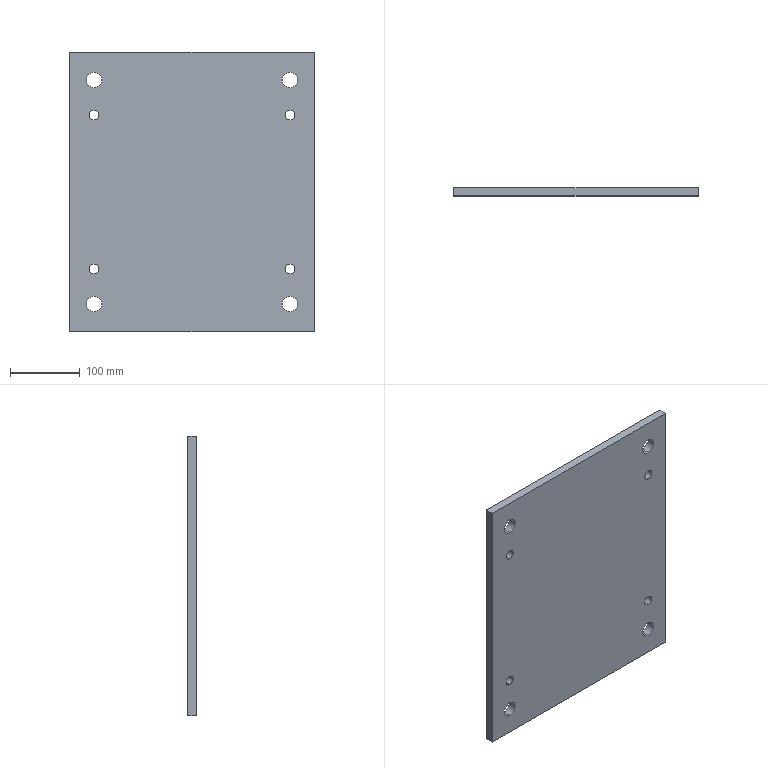Part | STEP file | 立柱底Plate-400×350 | 1 solid | 22 faces | box 350 x 12 x 400 mm | volume 1654365 mm3 | cylinder 16 | plane 6 | commonest cylinder face diameters 14 x8 22 x8